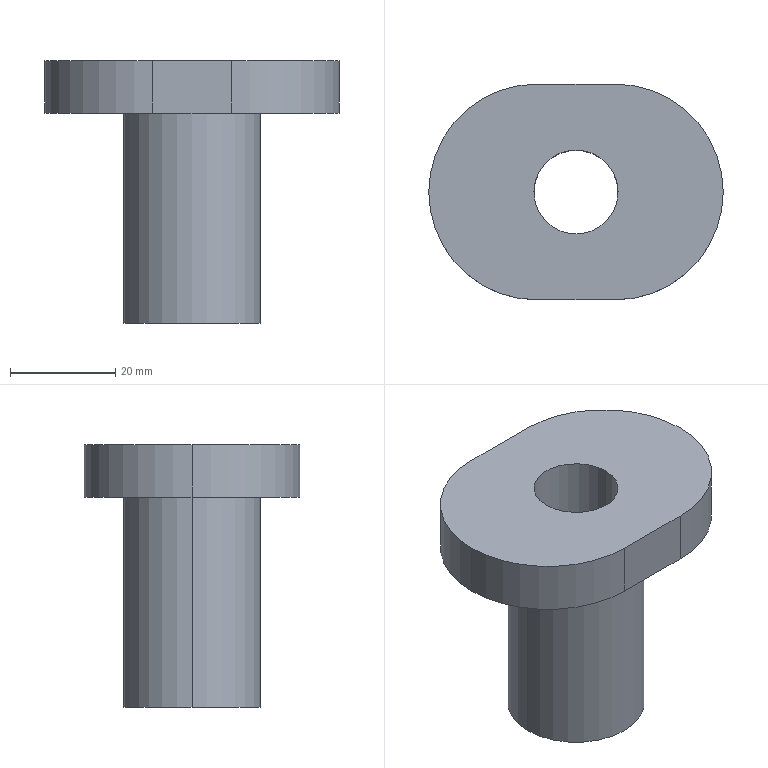Part | STEP file | ASND-0110-6.5aq | 1 solid | 12 faces | box 56 x 41 x 50 mm | volume 30537 mm3 | cylinder 7 | plane 5 | commonest cylinder face diameters 41 x3 16 x2 26 x2
STEP:
#1=CARTESIAN_POINT('',(0.,0.,0.));
#2=DIRECTION('',(0.,0.,1.));
#3=DIRECTION('',(1.,0.,0.));
#4=AXIS2_PLACEMENT_3D('',#1,#2,#3);
#5=CARTESIAN_POINT('',(-28.,0.,50.));
#6=VERTEX_POINT('',#5);
#7=CARTESIAN_POINT('',(-7.5,-20.5,50.));
#8=VERTEX_POINT('',#7);
#9=CARTESIAN_POINT('',(-7.5,0.,50.));
#10=DIRECTION('',(0.,0.,1.));
#11=DIRECTION('',(1.,0.,0.));
#12=AXIS2_PLACEMENT_3D('',#9,#10,#11);
#13=CIRCLE('',#12,20.5);
#14=CARTESIAN_POINT('',(-7.5,0.,50.));
#15=DIRECTION('',(0.,0.,-1.));
#16=DIRECTION('',(-1.,0.,0.));
#17=AXIS2_PLACEMENT_3D('',#14,#15,#16);
#18=CYLINDRICAL_SURFACE('',#17,20.5);
#19=CARTESIAN_POINT('',(9.425,0.));
#20=DIRECTION('',(-1.,0.));
#21=VECTOR('',#20,1.);
#22=LINE('',#19,#21);
#23=(GEOMETRIC_REPRESENTATION_CONTEXT(2)PARAMETRIC_REPRESENTATION_CONTEXT()REPRESENTATION_CONTEXT('',''));
#24=DEFINITIONAL_REPRESENTATION('',(#22),#23);
#25=PCURVE('',#18,#24);
#26=CARTESIAN_POINT('',(-7.5,0.,50.));
#27=DIRECTION('',(0.,0.,1.));
#28=DIRECTION('',(0.7071,0.7071,0.));
#29=AXIS2_PLACEMENT_3D('',#26,#27,#28);
#30=PLANE('',#29);
#31=CARTESIAN_POINT('',(0.,0.));
#32=DIRECTION('',(0.7071,-0.7071));
#33=AXIS2_PLACEMENT_2D('',#31,#32);
#34=CIRCLE('',#33,20.5);
#35=(GEOMETRIC_REPRESENTATION_CONTEXT(2)PARAMETRIC_REPRESENTATION_CONTEXT()REPRESENTATION_CONTEXT('',''));
#36=DEFINITIONAL_REPRESENTATION('',(#34),#35);
#37=PCURVE('',#30,#36);
#38=SURFACE_CURVE('',#13,(#25,#37),.PCURVE_S1.);
#39=EDGE_CURVE('',#6,#8,#38,.T.);
#40=ORIENTED_EDGE('',*,*,#39,.F.);
#41=CARTESIAN_POINT('',(-28.,0.,40.));
#42=VERTEX_POINT('',#41);
#43=CARTESIAN_POINT('',(-28.,0.,50.));
#44=DIRECTION('',(0.,0.,-1.));
#45=VECTOR('',#44,1.);
#46=LINE('',#43,#45);
#47=CARTESIAN_POINT('',(6.283,0.));
#48=DIRECTION('',(0.,1.));
#49=VECTOR('',#48,1.);
#50=LINE('',#47,#49);
#51=(GEOMETRIC_REPRESENTATION_CONTEXT(2)PARAMETRIC_REPRESENTATION_CONTEXT()REPRESENTATION_CONTEXT('',''));
#52=DEFINITIONAL_REPRESENTATION('',(#50),#51);
#53=PCURVE('',#18,#52);
#54=CARTESIAN_POINT('',(-7.5,0.,50.));
#55=DIRECTION('',(0.,0.,-1.));
#56=DIRECTION('',(-1.,0.,0.));
#57=AXIS2_PLACEMENT_3D('',#54,#55,#56);
#58=CYLINDRICAL_SURFACE('',#57,20.5);
#59=CARTESIAN_POINT('',(0.,0.));
#60=DIRECTION('',(0.,1.));
#61=VECTOR('',#60,1.);
#62=LINE('',#59,#61);
#63=(GEOMETRIC_REPRESENTATION_CONTEXT(2)PARAMETRIC_REPRESENTATION_CONTEXT()REPRESENTATION_CONTEXT('',''));
#64=DEFINITIONAL_REPRESENTATION('',(#62),#63);
#65=PCURVE('',#58,#64);
#66=SURFACE_CURVE('',#46,(#53,#65),.PCURVE_S1.);
#67=EDGE_CURVE('',#6,#42,#66,.T.);
#68=ORIENTED_EDGE('',*,*,#67,.T.);
#69=CARTESIAN_POINT('',(-7.5,-20.5,40.));
#70=VERTEX_POINT('',#69);
#71=CARTESIAN_POINT('',(-7.5,0.,40.));
#72=DIRECTION('',(0.,0.,1.));
#73=DIRECTION('',(1.,0.,0.));
#74=AXIS2_PLACEMENT_3D('',#71,#72,#73);
#75=CIRCLE('',#74,20.5);
#76=CARTESIAN_POINT('',(9.425,10.));
#77=DIRECTION('',(-1.,0.));
#78=VECTOR('',#77,1.);
#79=LINE('',#76,#78);
#80=(GEOMETRIC_REPRESENTATION_CONTEXT(2)PARAMETRIC_REPRESENTATION_CONTEXT()REPRESENTATION_CONTEXT('',''));
#81=DEFINITIONAL_REPRESENTATION('',(#79),#80);
#82=PCURVE('',#18,#81);
#83=CARTESIAN_POINT('',(-7.5,0.,40.));
#84=DIRECTION('',(0.,0.,1.));
#85=DIRECTION('',(0.7071,0.7071,0.));
#86=AXIS2_PLACEMENT_3D('',#83,#84,#85);
#87=PLANE('',#86);
#88=CARTESIAN_POINT('',(0.,0.));
#89=DIRECTION('',(0.7071,-0.7071));
#90=AXIS2_PLACEMENT_2D('',#88,#89);
#91=CIRCLE('',#90,20.5);
#92=(GEOMETRIC_REPRESENTATION_CONTEXT(2)PARAMETRIC_REPRESENTATION_CONTEXT()REPRESENTATION_CONTEXT('',''));
#93=DEFINITIONAL_REPRESENTATION('',(#91),#92);
#94=PCURVE('',#87,#93);
#95=SURFACE_CURVE('',#75,(#82,#94),.PCURVE_S1.);
#96=EDGE_CURVE('',#42,#70,#95,.T.);
#97=ORIENTED_EDGE('',*,*,#96,.T.);
#98=CARTESIAN_POINT('',(-7.5,-20.5,50.));
#99=DIRECTION('',(0.,0.,-1.));
#100=VECTOR('',#99,1.);
#101=LINE('',#98,#100);
#102=CARTESIAN_POINT('',(4.712,0.));
#103=DIRECTION('',(0.,1.));
#104=VECTOR('',#103,1.);
#105=LINE('',#102,#104);
#106=(GEOMETRIC_REPRESENTATION_CONTEXT(2)PARAMETRIC_REPRESENTATION_CONTEXT()REPRESENTATION_CONTEXT('',''));
#107=DEFINITIONAL_REPRESENTATION('',(#105),#106);
#108=PCURVE('',#18,#107);
#109=CARTESIAN_POINT('',(-7.5,-20.5,50.));
#110=DIRECTION('',(0.,1.,0.));
#111=DIRECTION('',(0.7071,0.,0.7071));
#112=AXIS2_PLACEMENT_3D('',#109,#110,#111);
#113=PLANE('',#112);
#114=CARTESIAN_POINT('',(0.,0.));
#115=DIRECTION('',(-0.7071,0.7071));
#116=VECTOR('',#115,1.);
#117=LINE('',#114,#116);
#118=(GEOMETRIC_REPRESENTATION_CONTEXT(2)PARAMETRIC_REPRESENTATION_CONTEXT()REPRESENTATION_CONTEXT('',''));
#119=DEFINITIONAL_REPRESENTATION('',(#117),#118);
#120=PCURVE('',#113,#119);
#121=SURFACE_CURVE('',#101,(#108,#120),.PCURVE_S1.);
#122=EDGE_CURVE('',#8,#70,#121,.T.);
#123=ORIENTED_EDGE('',*,*,#122,.F.);
#124=EDGE_LOOP('',(#40,#68,#97,#123));
#125=FACE_BOUND('',#124,.T.);
#126=ADVANCED_FACE('',(#125),#18,.T.);
#127=CARTESIAN_POINT('',(-8.,0.,50.));
#128=VERTEX_POINT('',#127);
#129=CARTESIAN_POINT('',(-8.,0.,0.));
#130=VERTEX_POINT('',#129);
#131=CARTESIAN_POINT('',(-8.,0.,40.));
#132=DIRECTION('',(0.,0.,-1.));
#133=VECTOR('',#132,1.);
#134=LINE('',#131,#133);
#135=CARTESIAN_POINT('',(0.,0.,40.));
#136=DIRECTION('',(0.,0.,-1.));
#137=DIRECTION('',(-1.,0.,0.));
#138=AXIS2_PLACEMENT_3D('',#135,#136,#137);
#139=CYLINDRICAL_SURFACE('',#138,8.);
#140=CARTESIAN_POINT('',(6.283,0.));
#141=DIRECTION('',(0.,1.));
#142=VECTOR('',#141,1.);
#143=LINE('',#140,#142);
#144=(GEOMETRIC_REPRESENTATION_CONTEXT(2)PARAMETRIC_REPRESENTATION_CONTEXT()REPRESENTATION_CONTEXT('',''));
#145=DEFINITIONAL_REPRESENTATION('',(#143),#144);
#146=PCURVE('',#139,#145);
#147=CARTESIAN_POINT('',(0.,0.,40.));
#148=DIRECTION('',(0.,0.,-1.));
#149=DIRECTION('',(-1.,0.,0.));
#150=AXIS2_PLACEMENT_3D('',#147,#148,#149);
#151=CYLINDRICAL_SURFACE('',#150,8.);
#152=CARTESIAN_POINT('',(0.,0.));
#153=DIRECTION('',(0.,1.));
#154=VECTOR('',#153,1.);
#155=LINE('',#152,#154);
#156=(GEOMETRIC_REPRESENTATION_CONTEXT(2)PARAMETRIC_REPRESENTATION_CONTEXT()REPRESENTATION_CONTEXT('',''));
#157=DEFINITIONAL_REPRESENTATION('',(#155),#156);
#158=PCURVE('',#151,#157);
#159=SURFACE_CURVE('',#134,(#146,#158),.PCURVE_S1.);
#160=EDGE_CURVE('',#128,#130,#159,.T.);
#161=ORIENTED_EDGE('',*,*,#160,.T.);
#162=CARTESIAN_POINT('',(8.,0.,0.));
#163=VERTEX_POINT('',#162);
#164=CARTESIAN_POINT('',(0.,0.,0.));
#165=DIRECTION('',(0.,0.,1.));
#166=DIRECTION('',(1.,0.,0.));
#167=AXIS2_PLACEMENT_3D('',#164,#165,#166);
#168=CIRCLE('',#167,8.);
#169=CARTESIAN_POINT('',(9.425,40.));
#170=DIRECTION('',(-1.,0.));
#171=VECTOR('',#170,1.);
#172=LINE('',#169,#171);
#173=(GEOMETRIC_REPRESENTATION_CONTEXT(2)PARAMETRIC_REPRESENTATION_CONTEXT()REPRESENTATION_CONTEXT('',''));
#174=DEFINITIONAL_REPRESENTATION('',(#172),#173);
#175=PCURVE('',#139,#174);
#176=CARTESIAN_POINT('',(0.,0.,0.));
#177=DIRECTION('',(0.,0.,1.));
#178=DIRECTION('',(0.7071,0.7071,0.));
#179=AXIS2_PLACEMENT_3D('',#176,#177,#178);
#180=PLANE('',#179);
#181=CARTESIAN_POINT('',(0.,0.));
#182=DIRECTION('',(0.7071,-0.7071));
#183=AXIS2_PLACEMENT_2D('',#181,#182);
#184=CIRCLE('',#183,8.);
#185=(GEOMETRIC_REPRESENTATION_CONTEXT(2)PARAMETRIC_REPRESENTATION_CONTEXT()REPRESENTATION_CONTEXT('',''));
#186=DEFINITIONAL_REPRESENTATION('',(#184),#185);
#187=PCURVE('',#180,#186);
#188=SURFACE_CURVE('',#168,(#175,#187),.PCURVE_S1.);
#189=EDGE_CURVE('',#130,#163,#188,.T.);
#190=ORIENTED_EDGE('',*,*,#189,.T.);
#191=CARTESIAN_POINT('',(8.,0.,50.));
#192=VERTEX_POINT('',#191);
#193=CARTESIAN_POINT('',(8.,0.,40.));
#194=DIRECTION('',(0.,0.,-1.));
#195=VECTOR('',#194,1.);
#196=LINE('',#193,#195);
#197=CARTESIAN_POINT('',(3.142,0.));
#198=DIRECTION('',(0.,1.));
#199=VECTOR('',#198,1.);
#200=LINE('',#197,#199);
#201=(GEOMETRIC_REPRESENTATION_CONTEXT(2)PARAMETRIC_REPRESENTATION_CONTEXT()REPRESENTATION_CONTEXT('',''));
#202=DEFINITIONAL_REPRESENTATION('',(#200),#201);
#203=PCURVE('',#139,#202);
#204=CARTESIAN_POINT('',(3.142,0.));
#205=DIRECTION('',(0.,1.));
#206=VECTOR('',#205,1.);
#207=LINE('',#204,#206);
#208=(GEOMETRIC_REPRESENTATION_CONTEXT(2)PARAMETRIC_REPRESENTATION_CONTEXT()REPRESENTATION_CONTEXT('',''));
#209=DEFINITIONAL_REPRESENTATION('',(#207),#208);
#210=PCURVE('',#151,#209);
#211=SURFACE_CURVE('',#196,(#203,#210),.PCURVE_S1.);
#212=EDGE_CURVE('',#192,#163,#211,.T.);
#213=ORIENTED_EDGE('',*,*,#212,.F.);
#214=CARTESIAN_POINT('',(0.,0.,50.));
#215=DIRECTION('',(0.,0.,1.));
#216=DIRECTION('',(1.,0.,0.));
#217=AXIS2_PLACEMENT_3D('',#214,#215,#216);
#218=CIRCLE('',#217,8.);
#219=CARTESIAN_POINT('',(9.425,-10.));
#220=DIRECTION('',(-1.,0.));
#221=VECTOR('',#220,1.);
#222=LINE('',#219,#221);
#223=(GEOMETRIC_REPRESENTATION_CONTEXT(2)PARAMETRIC_REPRESENTATION_CONTEXT()REPRESENTATION_CONTEXT('',''));
#224=DEFINITIONAL_REPRESENTATION('',(#222),#223);
#225=PCURVE('',#139,#224);
#226=CARTESIAN_POINT('',(5.303,-5.303));
#227=DIRECTION('',(0.7071,-0.7071));
#228=AXIS2_PLACEMENT_2D('',#226,#227);
#229=CIRCLE('',#228,8.);
#230=(GEOMETRIC_REPRESENTATION_CONTEXT(2)PARAMETRIC_REPRESENTATION_CONTEXT()REPRESENTATION_CONTEXT('',''));
#231=DEFINITIONAL_REPRESENTATION('',(#229),#230);
#232=PCURVE('',#30,#231);
#233=SURFACE_CURVE('',#218,(#225,#232),.PCURVE_S1.);
#234=EDGE_CURVE('',#128,#192,#233,.T.);
#235=ORIENTED_EDGE('',*,*,#234,.F.);
#236=EDGE_LOOP('',(#161,#190,#213,#235));
#237=FACE_BOUND('',#236,.F.);
#238=ADVANCED_FACE('',(#237),#139,.F.);
#239=CARTESIAN_POINT('',(13.,0.,40.));
#240=VERTEX_POINT('',#239);
#241=CARTESIAN_POINT('',(-13.,0.,40.));
#242=VERTEX_POINT('',#241);
#243=CARTESIAN_POINT('',(0.,0.,40.));
#244=DIRECTION('',(0.,0.,1.));
#245=DIRECTION('',(1.,0.,0.));
#246=AXIS2_PLACEMENT_3D('',#243,#244,#245);
#247=CIRCLE('',#246,13.);
#248=CARTESIAN_POINT('',(0.,0.,40.));
#249=DIRECTION('',(0.,0.,-1.));
#250=DIRECTION('',(-1.,0.,0.));
#251=AXIS2_PLACEMENT_3D('',#248,#249,#250);
#252=CYLINDRICAL_SURFACE('',#251,13.);
#253=CARTESIAN_POINT('',(3.142,0.));
#254=DIRECTION('',(-1.,0.));
#255=VECTOR('',#254,1.);
#256=LINE('',#253,#255);
#257=(GEOMETRIC_REPRESENTATION_CONTEXT(2)PARAMETRIC_REPRESENTATION_CONTEXT()REPRESENTATION_CONTEXT('',''));
#258=DEFINITIONAL_REPRESENTATION('',(#256),#257);
#259=PCURVE('',#252,#258);
#260=CARTESIAN_POINT('',(5.303,-5.303));
#261=DIRECTION('',(0.7071,-0.7071));
#262=AXIS2_PLACEMENT_2D('',#260,#261);
#263=CIRCLE('',#262,13.);
#264=(GEOMETRIC_REPRESENTATION_CONTEXT(2)PARAMETRIC_REPRESENTATION_CONTEXT()REPRESENTATION_CONTEXT('',''));
#265=DEFINITIONAL_REPRESENTATION('',(#263),#264);
#266=PCURVE('',#87,#265);
#267=SURFACE_CURVE('',#247,(#259,#266),.PCURVE_S1.);
#268=EDGE_CURVE('',#240,#242,#267,.T.);
#269=ORIENTED_EDGE('',*,*,#268,.F.);
#270=CARTESIAN_POINT('',(13.,0.,0.));
#271=VERTEX_POINT('',#270);
#272=CARTESIAN_POINT('',(13.,0.,40.));
#273=DIRECTION('',(0.,0.,-1.));
#274=VECTOR('',#273,1.);
#275=LINE('',#272,#274);
#276=CARTESIAN_POINT('',(3.142,0.));
#277=DIRECTION('',(0.,1.));
#278=VECTOR('',#277,1.);
#279=LINE('',#276,#278);
#280=(GEOMETRIC_REPRESENTATION_CONTEXT(2)PARAMETRIC_REPRESENTATION_CONTEXT()REPRESENTATION_CONTEXT('',''));
#281=DEFINITIONAL_REPRESENTATION('',(#279),#280);
#282=PCURVE('',#252,#281);
#283=CARTESIAN_POINT('',(0.,0.,40.));
#284=DIRECTION('',(0.,0.,-1.));
#285=DIRECTION('',(-1.,0.,0.));
#286=AXIS2_PLACEMENT_3D('',#283,#284,#285);
#287=CYLINDRICAL_SURFACE('',#286,13.);
#288=CARTESIAN_POINT('',(3.142,0.));
#289=DIRECTION('',(0.,1.));
#290=VECTOR('',#289,1.);
#291=LINE('',#288,#290);
#292=(GEOMETRIC_REPRESENTATION_CONTEXT(2)PARAMETRIC_REPRESENTATION_CONTEXT()REPRESENTATION_CONTEXT('',''));
#293=DEFINITIONAL_REPRESENTATION('',(#291),#292);
#294=PCURVE('',#287,#293);
#295=SURFACE_CURVE('',#275,(#282,#294),.PCURVE_S1.);
#296=EDGE_CURVE('',#240,#271,#295,.T.);
#297=ORIENTED_EDGE('',*,*,#296,.T.);
#298=CARTESIAN_POINT('',(-13.,0.,0.));
#299=VERTEX_POINT('',#298);
#300=CARTESIAN_POINT('',(0.,0.,0.));
#301=DIRECTION('',(0.,0.,1.));
#302=DIRECTION('',(1.,0.,0.));
#303=AXIS2_PLACEMENT_3D('',#300,#301,#302);
#304=CIRCLE('',#303,13.);
#305=CARTESIAN_POINT('',(3.142,40.));
#306=DIRECTION('',(-1.,0.));
#307=VECTOR('',#306,1.);
#308=LINE('',#305,#307);
#309=(GEOMETRIC_REPRESENTATION_CONTEXT(2)PARAMETRIC_REPRESENTATION_CONTEXT()REPRESENTATION_CONTEXT('',''));
#310=DEFINITIONAL_REPRESENTATION('',(#308),#309);
#311=PCURVE('',#252,#310);
#312=CARTESIAN_POINT('',(0.,0.));
#313=DIRECTION('',(0.7071,-0.7071));
#314=AXIS2_PLACEMENT_2D('',#312,#313);
#315=CIRCLE('',#314,13.);
#316=(GEOMETRIC_REPRESENTATION_CONTEXT(2)PARAMETRIC_REPRESENTATION_CONTEXT()REPRESENTATION_CONTEXT('',''));
#317=DEFINITIONAL_REPRESENTATION('',(#315),#316);
#318=PCURVE('',#180,#317);
#319=SURFACE_CURVE('',#304,(#311,#318),.PCURVE_S1.);
#320=EDGE_CURVE('',#271,#299,#319,.T.);
#321=ORIENTED_EDGE('',*,*,#320,.T.);
#322=CARTESIAN_POINT('',(-13.,0.,40.));
#323=DIRECTION('',(0.,0.,-1.));
#324=VECTOR('',#323,1.);
#325=LINE('',#322,#324);
#326=CARTESIAN_POINT('',(0.,0.));
#327=DIRECTION('',(0.,1.));
#328=VECTOR('',#327,1.);
#329=LINE('',#326,#328);
#330=(GEOMETRIC_REPRESENTATION_CONTEXT(2)PARAMETRIC_REPRESENTATION_CONTEXT()REPRESENTATION_CONTEXT('',''));
#331=DEFINITIONAL_REPRESENTATION('',(#329),#330);
#332=PCURVE('',#252,#331);
#333=CARTESIAN_POINT('',(6.283,0.));
#334=DIRECTION('',(0.,1.));
#335=VECTOR('',#334,1.);
#336=LINE('',#333,#335);
#337=(GEOMETRIC_REPRESENTATION_CONTEXT(2)PARAMETRIC_REPRESENTATION_CONTEXT()REPRESENTATION_CONTEXT('',''));
#338=DEFINITIONAL_REPRESENTATION('',(#336),#337);
#339=PCURVE('',#287,#338);
#340=SURFACE_CURVE('',#325,(#332,#339),.PCURVE_S1.);
#341=EDGE_CURVE('',#242,#299,#340,.T.);
#342=ORIENTED_EDGE('',*,*,#341,.F.);
#343=EDGE_LOOP('',(#269,#297,#321,#342));
#344=FACE_BOUND('',#343,.T.);
#345=ADVANCED_FACE('',(#344),#252,.T.);
#346=CARTESIAN_POINT('',(0.,0.,0.));
#347=DIRECTION('',(0.,0.,1.));
#348=DIRECTION('',(1.,0.,0.));
#349=AXIS2_PLACEMENT_3D('',#346,#347,#348);
#350=CIRCLE('',#349,13.);
#351=CARTESIAN_POINT('',(0.,0.));
#352=DIRECTION('',(0.7071,-0.7071));
#353=AXIS2_PLACEMENT_2D('',#351,#352);
#354=CIRCLE('',#353,13.);
#355=(GEOMETRIC_REPRESENTATION_CONTEXT(2)PARAMETRIC_REPRESENTATION_CONTEXT()REPRESENTATION_CONTEXT('',''));
#356=DEFINITIONAL_REPRESENTATION('',(#354),#355);
#357=PCURVE('',#180,#356);
#358=CARTESIAN_POINT('',(9.425,40.));
#359=DIRECTION('',(-1.,0.));
#360=VECTOR('',#359,1.);
#361=LINE('',#358,#360);
#362=(GEOMETRIC_REPRESENTATION_CONTEXT(2)PARAMETRIC_REPRESENTATION_CONTEXT()REPRESENTATION_CONTEXT('',''));
#363=DEFINITIONAL_REPRESENTATION('',(#361),#362);
#364=PCURVE('',#287,#363);
#365=SURFACE_CURVE('',#350,(#357,#364),.PCURVE_S1.);
#366=EDGE_CURVE('',#299,#271,#365,.T.);
#367=ORIENTED_EDGE('',*,*,#366,.F.);
#368=ORIENTED_EDGE('',*,*,#320,.F.);
#369=EDGE_LOOP('',(#367,#368));
#370=FACE_BOUND('',#369,.T.);
#371=ORIENTED_EDGE('',*,*,#189,.T.);
#372=CARTESIAN_POINT('',(0.,0.,0.));
#373=DIRECTION('',(0.,0.,1.));
#374=DIRECTION('',(1.,0.,0.));
#375=AXIS2_PLACEMENT_3D('',#372,#373,#374);
#376=CIRCLE('',#375,8.);
#377=CARTESIAN_POINT('',(0.,0.));
#378=DIRECTION('',(0.7071,-0.7071));
#379=AXIS2_PLACEMENT_2D('',#377,#378);
#380=CIRCLE('',#379,8.);
#381=(GEOMETRIC_REPRESENTATION_CONTEXT(2)PARAMETRIC_REPRESENTATION_CONTEXT()REPRESENTATION_CONTEXT('',''));
#382=DEFINITIONAL_REPRESENTATION('',(#380),#381);
#383=PCURVE('',#180,#382);
#384=CARTESIAN_POINT('',(3.142,40.));
#385=DIRECTION('',(-1.,0.));
#386=VECTOR('',#385,1.);
#387=LINE('',#384,#386);
#388=(GEOMETRIC_REPRESENTATION_CONTEXT(2)PARAMETRIC_REPRESENTATION_CONTEXT()REPRESENTATION_CONTEXT('',''));
#389=DEFINITIONAL_REPRESENTATION('',(#387),#388);
#390=PCURVE('',#151,#389);
#391=SURFACE_CURVE('',#376,(#383,#390),.PCURVE_S1.);
#392=EDGE_CURVE('',#163,#130,#391,.T.);
#393=ORIENTED_EDGE('',*,*,#392,.T.);
#394=EDGE_LOOP('',(#371,#393));
#395=FACE_BOUND('',#394,.T.);
#396=ADVANCED_FACE('',(#370,#395),#180,.F.);
#397=ORIENTED_EDGE('',*,*,#296,.F.);
#398=CARTESIAN_POINT('',(0.,0.,40.));
#399=DIRECTION('',(0.,0.,1.));
#400=DIRECTION('',(1.,0.,0.));
#401=AXIS2_PLACEMENT_3D('',#398,#399,#400);
#402=CIRCLE('',#401,13.);
#403=CARTESIAN_POINT('',(9.425,0.));
#404=DIRECTION('',(-1.,0.));
#405=VECTOR('',#404,1.);
#406=LINE('',#403,#405);
#407=(GEOMETRIC_REPRESENTATION_CONTEXT(2)PARAMETRIC_REPRESENTATION_CONTEXT()REPRESENTATION_CONTEXT('',''));
#408=DEFINITIONAL_REPRESENTATION('',(#406),#407);
#409=PCURVE('',#287,#408);
#410=CARTESIAN_POINT('',(5.303,-5.303));
#411=DIRECTION('',(0.7071,-0.7071));
#412=AXIS2_PLACEMENT_2D('',#410,#411);
#413=CIRCLE('',#412,13.);
#414=(GEOMETRIC_REPRESENTATION_CONTEXT(2)PARAMETRIC_REPRESENTATION_CONTEXT()REPRESENTATION_CONTEXT('',''));
#415=DEFINITIONAL_REPRESENTATION('',(#413),#414);
#416=PCURVE('',#87,#415);
#417=SURFACE_CURVE('',#402,(#409,#416),.PCURVE_S1.);
#418=EDGE_CURVE('',#242,#240,#417,.T.);
#419=ORIENTED_EDGE('',*,*,#418,.F.);
#420=ORIENTED_EDGE('',*,*,#341,.T.);
#421=ORIENTED_EDGE('',*,*,#366,.T.);
#422=EDGE_LOOP('',(#397,#419,#420,#421));
#423=FACE_BOUND('',#422,.T.);
#424=ADVANCED_FACE('',(#423),#287,.T.);
#425=ORIENTED_EDGE('',*,*,#392,.T.);
#426=ORIENTED_EDGE('',*,*,#160,.F.);
#427=CARTESIAN_POINT('',(0.,0.,50.));
#428=DIRECTION('',(0.,0.,1.));
#429=DIRECTION('',(1.,0.,0.));
#430=AXIS2_PLACEMENT_3D('',#427,#428,#429);
#431=CIRCLE('',#430,8.);
#432=CARTESIAN_POINT('',(3.142,-10.));
#433=DIRECTION('',(-1.,0.));
#434=VECTOR('',#433,1.);
#435=LINE('',#432,#434);
#436=(GEOMETRIC_REPRESENTATION_CONTEXT(2)PARAMETRIC_REPRESENTATION_CONTEXT()REPRESENTATION_CONTEXT('',''));
#437=DEFINITIONAL_REPRESENTATION('',(#435),#436);
#438=PCURVE('',#151,#437);
#439=CARTESIAN_POINT('',(5.303,-5.303));
#440=DIRECTION('',(0.7071,-0.7071));
#441=AXIS2_PLACEMENT_2D('',#439,#440);
#442=CIRCLE('',#441,8.);
#443=(GEOMETRIC_REPRESENTATION_CONTEXT(2)PARAMETRIC_REPRESENTATION_CONTEXT()REPRESENTATION_CONTEXT('',''));
#444=DEFINITIONAL_REPRESENTATION('',(#442),#443);
#445=PCURVE('',#30,#444);
#446=SURFACE_CURVE('',#431,(#438,#445),.PCURVE_S1.);
#447=EDGE_CURVE('',#192,#128,#446,.T.);
#448=ORIENTED_EDGE('',*,*,#447,.F.);
#449=ORIENTED_EDGE('',*,*,#212,.T.);
#450=EDGE_LOOP('',(#425,#426,#448,#449));
#451=FACE_BOUND('',#450,.F.);
#452=ADVANCED_FACE('',(#451),#151,.F.);
#453=CARTESIAN_POINT('',(-7.5,20.5,40.));
#454=VERTEX_POINT('',#453);
#455=CARTESIAN_POINT('',(-7.5,0.,40.));
#456=DIRECTION('',(0.,0.,1.));
#457=DIRECTION('',(1.,0.,0.));
#458=AXIS2_PLACEMENT_3D('',#455,#456,#457);
#459=CIRCLE('',#458,20.5);
#460=CARTESIAN_POINT('',(0.,0.));
#461=DIRECTION('',(0.7071,-0.7071));
#462=AXIS2_PLACEMENT_2D('',#460,#461);
#463=CIRCLE('',#462,20.5);
#464=(GEOMETRIC_REPRESENTATION_CONTEXT(2)PARAMETRIC_REPRESENTATION_CONTEXT()REPRESENTATION_CONTEXT('',''));
#465=DEFINITIONAL_REPRESENTATION('',(#463),#464);
#466=PCURVE('',#87,#465);
#467=CARTESIAN_POINT('',(3.142,10.));
#468=DIRECTION('',(-1.,0.));
#469=VECTOR('',#468,1.);
#470=LINE('',#467,#469);
#471=(GEOMETRIC_REPRESENTATION_CONTEXT(2)PARAMETRIC_REPRESENTATION_CONTEXT()REPRESENTATION_CONTEXT('',''));
#472=DEFINITIONAL_REPRESENTATION('',(#470),#471);
#473=PCURVE('',#58,#472);
#474=SURFACE_CURVE('',#459,(#466,#473),.PCURVE_S1.);
#475=EDGE_CURVE('',#454,#42,#474,.T.);
#476=ORIENTED_EDGE('',*,*,#475,.F.);
#477=CARTESIAN_POINT('',(7.5,20.5,40.));
#478=VERTEX_POINT('',#477);
#479=CARTESIAN_POINT('',(7.5,20.5,40.));
#480=DIRECTION('',(-1.,0.,0.));
#481=VECTOR('',#480,1.);
#482=LINE('',#479,#481);
#483=CARTESIAN_POINT('',(25.102,3.889));
#484=DIRECTION('',(-0.7071,0.7071));
#485=VECTOR('',#484,1.);
#486=LINE('',#483,#485);
#487=(GEOMETRIC_REPRESENTATION_CONTEXT(2)PARAMETRIC_REPRESENTATION_CONTEXT()REPRESENTATION_CONTEXT('',''));
#488=DEFINITIONAL_REPRESENTATION('',(#486),#487);
#489=PCURVE('',#87,#488);
#490=CARTESIAN_POINT('',(-7.5,20.5,50.));
#491=DIRECTION('',(0.,-1.,0.));
#492=DIRECTION('',(0.7071,0.,0.7071));
#493=AXIS2_PLACEMENT_3D('',#490,#491,#492);
#494=PLANE('',#493);
#495=CARTESIAN_POINT('',(3.536,-17.678));
#496=DIRECTION('',(-0.7071,0.7071));
#497=VECTOR('',#496,1.);
#498=LINE('',#495,#497);
#499=(GEOMETRIC_REPRESENTATION_CONTEXT(2)PARAMETRIC_REPRESENTATION_CONTEXT()REPRESENTATION_CONTEXT('',''));
#500=DEFINITIONAL_REPRESENTATION('',(#498),#499);
#501=PCURVE('',#494,#500);
#502=SURFACE_CURVE('',#482,(#489,#501),.PCURVE_S1.);
#503=EDGE_CURVE('',#478,#454,#502,.T.);
#504=ORIENTED_EDGE('',*,*,#503,.F.);
#505=CARTESIAN_POINT('',(7.5,-20.5,40.));
#506=VERTEX_POINT('',#505);
#507=CARTESIAN_POINT('',(7.5,0.,40.));
#508=DIRECTION('',(0.,0.,1.));
#509=DIRECTION('',(1.,0.,0.));
#510=AXIS2_PLACEMENT_3D('',#507,#508,#509);
#511=CIRCLE('',#510,20.5);
#512=CARTESIAN_POINT('',(10.607,-10.607));
#513=DIRECTION('',(0.7071,-0.7071));
#514=AXIS2_PLACEMENT_2D('',#512,#513);
#515=CIRCLE('',#514,20.5);
#516=(GEOMETRIC_REPRESENTATION_CONTEXT(2)PARAMETRIC_REPRESENTATION_CONTEXT()REPRESENTATION_CONTEXT('',''));
#517=DEFINITIONAL_REPRESENTATION('',(#515),#516);
#518=PCURVE('',#87,#517);
#519=CARTESIAN_POINT('',(7.5,0.,50.));
#520=DIRECTION('',(0.,0.,-1.));
#521=DIRECTION('',(-1.,0.,0.));
#522=AXIS2_PLACEMENT_3D('',#519,#520,#521);
#523=CYLINDRICAL_SURFACE('',#522,20.5);
#524=CARTESIAN_POINT('',(9.425,10.));
#525=DIRECTION('',(-1.,0.));
#526=VECTOR('',#525,1.);
#527=LINE('',#524,#526);
#528=(GEOMETRIC_REPRESENTATION_CONTEXT(2)PARAMETRIC_REPRESENTATION_CONTEXT()REPRESENTATION_CONTEXT('',''));
#529=DEFINITIONAL_REPRESENTATION('',(#527),#528);
#530=PCURVE('',#523,#529);
#531=SURFACE_CURVE('',#511,(#518,#530),.PCURVE_S1.);
#532=EDGE_CURVE('',#506,#478,#531,.T.);
#533=ORIENTED_EDGE('',*,*,#532,.F.);
#534=CARTESIAN_POINT('',(-7.5,-20.5,40.));
#535=DIRECTION('',(1.,0.,0.));
#536=VECTOR('',#535,1.);
#537=LINE('',#534,#536);
#538=CARTESIAN_POINT('',(-14.496,-14.496));
#539=DIRECTION('',(0.7071,-0.7071));
#540=VECTOR('',#539,1.);
#541=LINE('',#538,#540);
#542=(GEOMETRIC_REPRESENTATION_CONTEXT(2)PARAMETRIC_REPRESENTATION_CONTEXT()REPRESENTATION_CONTEXT('',''));
#543=DEFINITIONAL_REPRESENTATION('',(#541),#542);
#544=PCURVE('',#87,#543);
#545=CARTESIAN_POINT('',(-7.071,7.071));
#546=DIRECTION('',(0.7071,0.7071));
#547=VECTOR('',#546,1.);
#548=LINE('',#545,#547);
#549=(GEOMETRIC_REPRESENTATION_CONTEXT(2)PARAMETRIC_REPRESENTATION_CONTEXT()REPRESENTATION_CONTEXT('',''));
#550=DEFINITIONAL_REPRESENTATION('',(#548),#549);
#551=PCURVE('',#113,#550);
#552=SURFACE_CURVE('',#537,(#544,#551),.PCURVE_S1.);
#553=EDGE_CURVE('',#70,#506,#552,.T.);
#554=ORIENTED_EDGE('',*,*,#553,.F.);
#555=ORIENTED_EDGE('',*,*,#96,.F.);
#556=EDGE_LOOP('',(#476,#504,#533,#554,#555));
#557=FACE_BOUND('',#556,.T.);
#558=ORIENTED_EDGE('',*,*,#418,.T.);
#559=ORIENTED_EDGE('',*,*,#268,.T.);
#560=EDGE_LOOP('',(#558,#559));
#561=FACE_BOUND('',#560,.T.);
#562=ADVANCED_FACE('',(#557,#561),#87,.F.);
#563=CARTESIAN_POINT('',(-7.5,20.5,50.));
#564=VERTEX_POINT('',#563);
#565=CARTESIAN_POINT('',(-7.5,0.,50.));
#566=DIRECTION('',(0.,0.,1.));
#567=DIRECTION('',(1.,0.,0.));
#568=AXIS2_PLACEMENT_3D('',#565,#566,#567);
#569=CIRCLE('',#568,20.5);
#570=CARTESIAN_POINT('',(0.,0.));
#571=DIRECTION('',(0.7071,-0.7071));
#572=AXIS2_PLACEMENT_2D('',#570,#571);
#573=CIRCLE('',#572,20.5);
#574=(GEOMETRIC_REPRESENTATION_CONTEXT(2)PARAMETRIC_REPRESENTATION_CONTEXT()REPRESENTATION_CONTEXT('',''));
#575=DEFINITIONAL_REPRESENTATION('',(#573),#574);
#576=PCURVE('',#30,#575);
#577=CARTESIAN_POINT('',(3.142,0.));
#578=DIRECTION('',(-1.,0.));
#579=VECTOR('',#578,1.);
#580=LINE('',#577,#579);
#581=(GEOMETRIC_REPRESENTATION_CONTEXT(2)PARAMETRIC_REPRESENTATION_CONTEXT()REPRESENTATION_CONTEXT('',''));
#582=DEFINITIONAL_REPRESENTATION('',(#580),#581);
#583=PCURVE('',#58,#582);
#584=SURFACE_CURVE('',#569,(#576,#583),.PCURVE_S1.);
#585=EDGE_CURVE('',#564,#6,#584,.T.);
#586=ORIENTED_EDGE('',*,*,#585,.T.);
#587=ORIENTED_EDGE('',*,*,#39,.T.);
#588=CARTESIAN_POINT('',(7.5,-20.5,50.));
#589=VERTEX_POINT('',#588);
#590=CARTESIAN_POINT('',(-7.5,-20.5,50.));
#591=DIRECTION('',(1.,0.,0.));
#592=VECTOR('',#591,1.);
#593=LINE('',#590,#592);
#594=CARTESIAN_POINT('',(-14.496,-14.496));
#595=DIRECTION('',(0.7071,-0.7071));
#596=VECTOR('',#595,1.);
#597=LINE('',#594,#596);
#598=(GEOMETRIC_REPRESENTATION_CONTEXT(2)PARAMETRIC_REPRESENTATION_CONTEXT()REPRESENTATION_CONTEXT('',''));
#599=DEFINITIONAL_REPRESENTATION('',(#597),#598);
#600=PCURVE('',#30,#599);
#601=CARTESIAN_POINT('',(0.,0.));
#602=DIRECTION('',(0.7071,0.7071));
#603=VECTOR('',#602,1.);
#604=LINE('',#601,#603);
#605=(GEOMETRIC_REPRESENTATION_CONTEXT(2)PARAMETRIC_REPRESENTATION_CONTEXT()REPRESENTATION_CONTEXT('',''));
#606=DEFINITIONAL_REPRESENTATION('',(#604),#605);
#607=PCURVE('',#113,#606);
#608=SURFACE_CURVE('',#593,(#600,#607),.PCURVE_S1.);
#609=EDGE_CURVE('',#8,#589,#608,.T.);
#610=ORIENTED_EDGE('',*,*,#609,.T.);
#611=CARTESIAN_POINT('',(7.5,20.5,50.));
#612=VERTEX_POINT('',#611);
#613=CARTESIAN_POINT('',(7.5,0.,50.));
#614=DIRECTION('',(0.,0.,1.));
#615=DIRECTION('',(1.,0.,0.));
#616=AXIS2_PLACEMENT_3D('',#613,#614,#615);
#617=CIRCLE('',#616,20.5);
#618=CARTESIAN_POINT('',(10.607,-10.607));
#619=DIRECTION('',(0.7071,-0.7071));
#620=AXIS2_PLACEMENT_2D('',#618,#619);
#621=CIRCLE('',#620,20.5);
#622=(GEOMETRIC_REPRESENTATION_CONTEXT(2)PARAMETRIC_REPRESENTATION_CONTEXT()REPRESENTATION_CONTEXT('',''));
#623=DEFINITIONAL_REPRESENTATION('',(#621),#622);
#624=PCURVE('',#30,#623);
#625=CARTESIAN_POINT('',(9.425,0.));
#626=DIRECTION('',(-1.,0.));
#627=VECTOR('',#626,1.);
#628=LINE('',#625,#627);
#629=(GEOMETRIC_REPRESENTATION_CONTEXT(2)PARAMETRIC_REPRESENTATION_CONTEXT()REPRESENTATION_CONTEXT('',''));
#630=DEFINITIONAL_REPRESENTATION('',(#628),#629);
#631=PCURVE('',#523,#630);
#632=SURFACE_CURVE('',#617,(#624,#631),.PCURVE_S1.);
#633=EDGE_CURVE('',#589,#612,#632,.T.);
#634=ORIENTED_EDGE('',*,*,#633,.T.);
#635=CARTESIAN_POINT('',(7.5,20.5,50.));
#636=DIRECTION('',(-1.,0.,0.));
#637=VECTOR('',#636,1.);
#638=LINE('',#635,#637);
#639=CARTESIAN_POINT('',(25.102,3.889));
#640=DIRECTION('',(-0.7071,0.7071));
#641=VECTOR('',#640,1.);
#642=LINE('',#639,#641);
#643=(GEOMETRIC_REPRESENTATION_CONTEXT(2)PARAMETRIC_REPRESENTATION_CONTEXT()REPRESENTATION_CONTEXT('',''));
#644=DEFINITIONAL_REPRESENTATION('',(#642),#643);
#645=PCURVE('',#30,#644);
#646=CARTESIAN_POINT('',(10.607,-10.607));
#647=DIRECTION('',(-0.7071,0.7071));
#648=VECTOR('',#647,1.);
#649=LINE('',#646,#648);
#650=(GEOMETRIC_REPRESENTATION_CONTEXT(2)PARAMETRIC_REPRESENTATION_CONTEXT()REPRESENTATION_CONTEXT('',''));
#651=DEFINITIONAL_REPRESENTATION('',(#649),#650);
#652=PCURVE('',#494,#651);
#653=SURFACE_CURVE('',#638,(#645,#652),.PCURVE_S1.);
#654=EDGE_CURVE('',#612,#564,#653,.T.);
#655=ORIENTED_EDGE('',*,*,#654,.T.);
#656=EDGE_LOOP('',(#586,#587,#610,#634,#655));
#657=FACE_BOUND('',#656,.T.);
#658=ORIENTED_EDGE('',*,*,#234,.F.);
#659=ORIENTED_EDGE('',*,*,#447,.F.);
#660=EDGE_LOOP('',(#658,#659));
#661=FACE_BOUND('',#660,.T.);
#662=ADVANCED_FACE('',(#657,#661),#30,.T.);
#663=ORIENTED_EDGE('',*,*,#67,.F.);
#664=ORIENTED_EDGE('',*,*,#585,.F.);
#665=CARTESIAN_POINT('',(-7.5,20.5,50.));
#666=DIRECTION('',(0.,0.,-1.));
#667=VECTOR('',#666,1.);
#668=LINE('',#665,#667);
#669=CARTESIAN_POINT('',(1.571,0.));
#670=DIRECTION('',(0.,1.));
#671=VECTOR('',#670,1.);
#672=LINE('',#669,#671);
#673=(GEOMETRIC_REPRESENTATION_CONTEXT(2)PARAMETRIC_REPRESENTATION_CONTEXT()REPRESENTATION_CONTEXT('',''));
#674=DEFINITIONAL_REPRESENTATION('',(#672),#673);
#675=PCURVE('',#58,#674);
#676=CARTESIAN_POINT('',(0.,0.));
#677=DIRECTION('',(-0.7071,-0.7071));
#678=VECTOR('',#677,1.);
#679=LINE('',#676,#678);
#680=(GEOMETRIC_REPRESENTATION_CONTEXT(2)PARAMETRIC_REPRESENTATION_CONTEXT()REPRESENTATION_CONTEXT('',''));
#681=DEFINITIONAL_REPRESENTATION('',(#679),#680);
#682=PCURVE('',#494,#681);
#683=SURFACE_CURVE('',#668,(#675,#682),.PCURVE_S1.);
#684=EDGE_CURVE('',#564,#454,#683,.T.);
#685=ORIENTED_EDGE('',*,*,#684,.T.);
#686=ORIENTED_EDGE('',*,*,#475,.T.);
#687=EDGE_LOOP('',(#663,#664,#685,#686));
#688=FACE_BOUND('',#687,.T.);
#689=ADVANCED_FACE('',(#688),#58,.T.);
#690=ORIENTED_EDGE('',*,*,#553,.T.);
#691=CARTESIAN_POINT('',(7.5,-20.5,50.));
#692=DIRECTION('',(0.,0.,-1.));
#693=VECTOR('',#692,1.);
#694=LINE('',#691,#693);
#695=CARTESIAN_POINT('',(10.607,10.607));
#696=DIRECTION('',(-0.7071,0.7071));
#697=VECTOR('',#696,1.);
#698=LINE('',#695,#697);
#699=(GEOMETRIC_REPRESENTATION_CONTEXT(2)PARAMETRIC_REPRESENTATION_CONTEXT()REPRESENTATION_CONTEXT('',''));
#700=DEFINITIONAL_REPRESENTATION('',(#698),#699);
#701=PCURVE('',#113,#700);
#702=CARTESIAN_POINT('',(4.712,0.));
#703=DIRECTION('',(0.,1.));
#704=VECTOR('',#703,1.);
#705=LINE('',#702,#704);
#706=(GEOMETRIC_REPRESENTATION_CONTEXT(2)PARAMETRIC_REPRESENTATION_CONTEXT()REPRESENTATION_CONTEXT('',''));
#707=DEFINITIONAL_REPRESENTATION('',(#705),#706);
#708=PCURVE('',#523,#707);
#709=SURFACE_CURVE('',#694,(#701,#708),.PCURVE_S1.);
#710=EDGE_CURVE('',#589,#506,#709,.T.);
#711=ORIENTED_EDGE('',*,*,#710,.F.);
#712=ORIENTED_EDGE('',*,*,#609,.F.);
#713=ORIENTED_EDGE('',*,*,#122,.T.);
#714=EDGE_LOOP('',(#690,#711,#712,#713));
#715=FACE_BOUND('',#714,.T.);
#716=ADVANCED_FACE('',(#715),#113,.F.);
#717=ORIENTED_EDGE('',*,*,#532,.T.);
#718=CARTESIAN_POINT('',(7.5,20.5,50.));
#719=DIRECTION('',(0.,0.,-1.));
#720=VECTOR('',#719,1.);
#721=LINE('',#718,#720);
#722=CARTESIAN_POINT('',(1.571,0.));
#723=DIRECTION('',(0.,1.));
#724=VECTOR('',#723,1.);
#725=LINE('',#722,#724);
#726=(GEOMETRIC_REPRESENTATION_CONTEXT(2)PARAMETRIC_REPRESENTATION_CONTEXT()REPRESENTATION_CONTEXT('',''));
#727=DEFINITIONAL_REPRESENTATION('',(#725),#726);
#728=PCURVE('',#523,#727);
#729=CARTESIAN_POINT('',(10.607,-10.607));
#730=DIRECTION('',(-0.7071,-0.7071));
#731=VECTOR('',#730,1.);
#732=LINE('',#729,#731);
#733=(GEOMETRIC_REPRESENTATION_CONTEXT(2)PARAMETRIC_REPRESENTATION_CONTEXT()REPRESENTATION_CONTEXT('',''));
#734=DEFINITIONAL_REPRESENTATION('',(#732),#733);
#735=PCURVE('',#494,#734);
#736=SURFACE_CURVE('',#721,(#728,#735),.PCURVE_S1.);
#737=EDGE_CURVE('',#612,#478,#736,.T.);
#738=ORIENTED_EDGE('',*,*,#737,.F.);
#739=ORIENTED_EDGE('',*,*,#633,.F.);
#740=ORIENTED_EDGE('',*,*,#710,.T.);
#741=EDGE_LOOP('',(#717,#738,#739,#740));
#742=FACE_BOUND('',#741,.T.);
#743=ADVANCED_FACE('',(#742),#523,.T.);
#744=ORIENTED_EDGE('',*,*,#503,.T.);
#745=ORIENTED_EDGE('',*,*,#684,.F.);
#746=ORIENTED_EDGE('',*,*,#654,.F.);
#747=ORIENTED_EDGE('',*,*,#737,.T.);
#748=EDGE_LOOP('',(#744,#745,#746,#747));
#749=FACE_BOUND('',#748,.T.);
#750=ADVANCED_FACE('',(#749),#494,.F.);
#751=CLOSED_SHELL('',(#126,#238,#345,#396,#424,#452,#562,#662,#689,#716,#743,#750));
#752=MANIFOLD_SOLID_BREP('',#751);
#753=(LENGTH_UNIT()NAMED_UNIT(*)SI_UNIT(.MILLI.,.METRE.));
#754=UNCERTAINTY_MEASURE_WITH_UNIT(LENGTH_MEASURE(0.0000001),#753,'','');
#755=(NAMED_UNIT(*)PLANE_ANGLE_UNIT()SI_UNIT($,.RADIAN.));
#756=(NAMED_UNIT(*)SI_UNIT($,.STERADIAN.)SOLID_ANGLE_UNIT());
#757=(GEOMETRIC_REPRESENTATION_CONTEXT(3)GLOBAL_UNCERTAINTY_ASSIGNED_CONTEXT((#754))GLOBAL_UNIT_ASSIGNED_CONTEXT((#753,#755,#756))REPRESENTATION_CONTEXT('',''));
#758=ADVANCED_BREP_SHAPE_REPRESENTATION('',(#4,#752),#757);